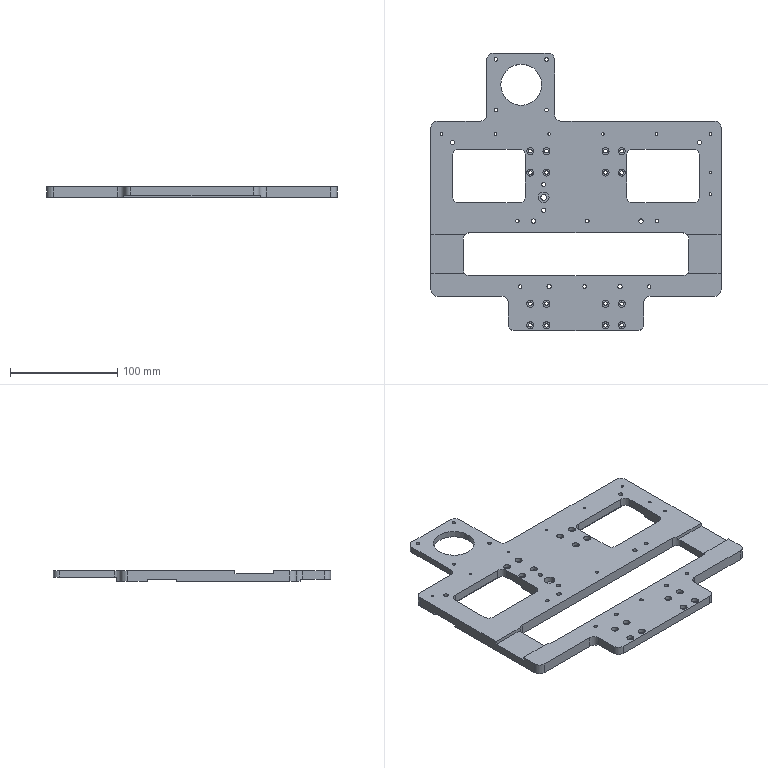Part | STEP file | QA-AD03 | 1 solid | 206 faces | box 270 x 258 x 10 mm | volume 320540 mm3 | cylinder 146 | plane 60 | commonest cylinder face diameters 3.4 x32 6.5 x32 12 x24 3.3 x20 2.5 x16 4 x16